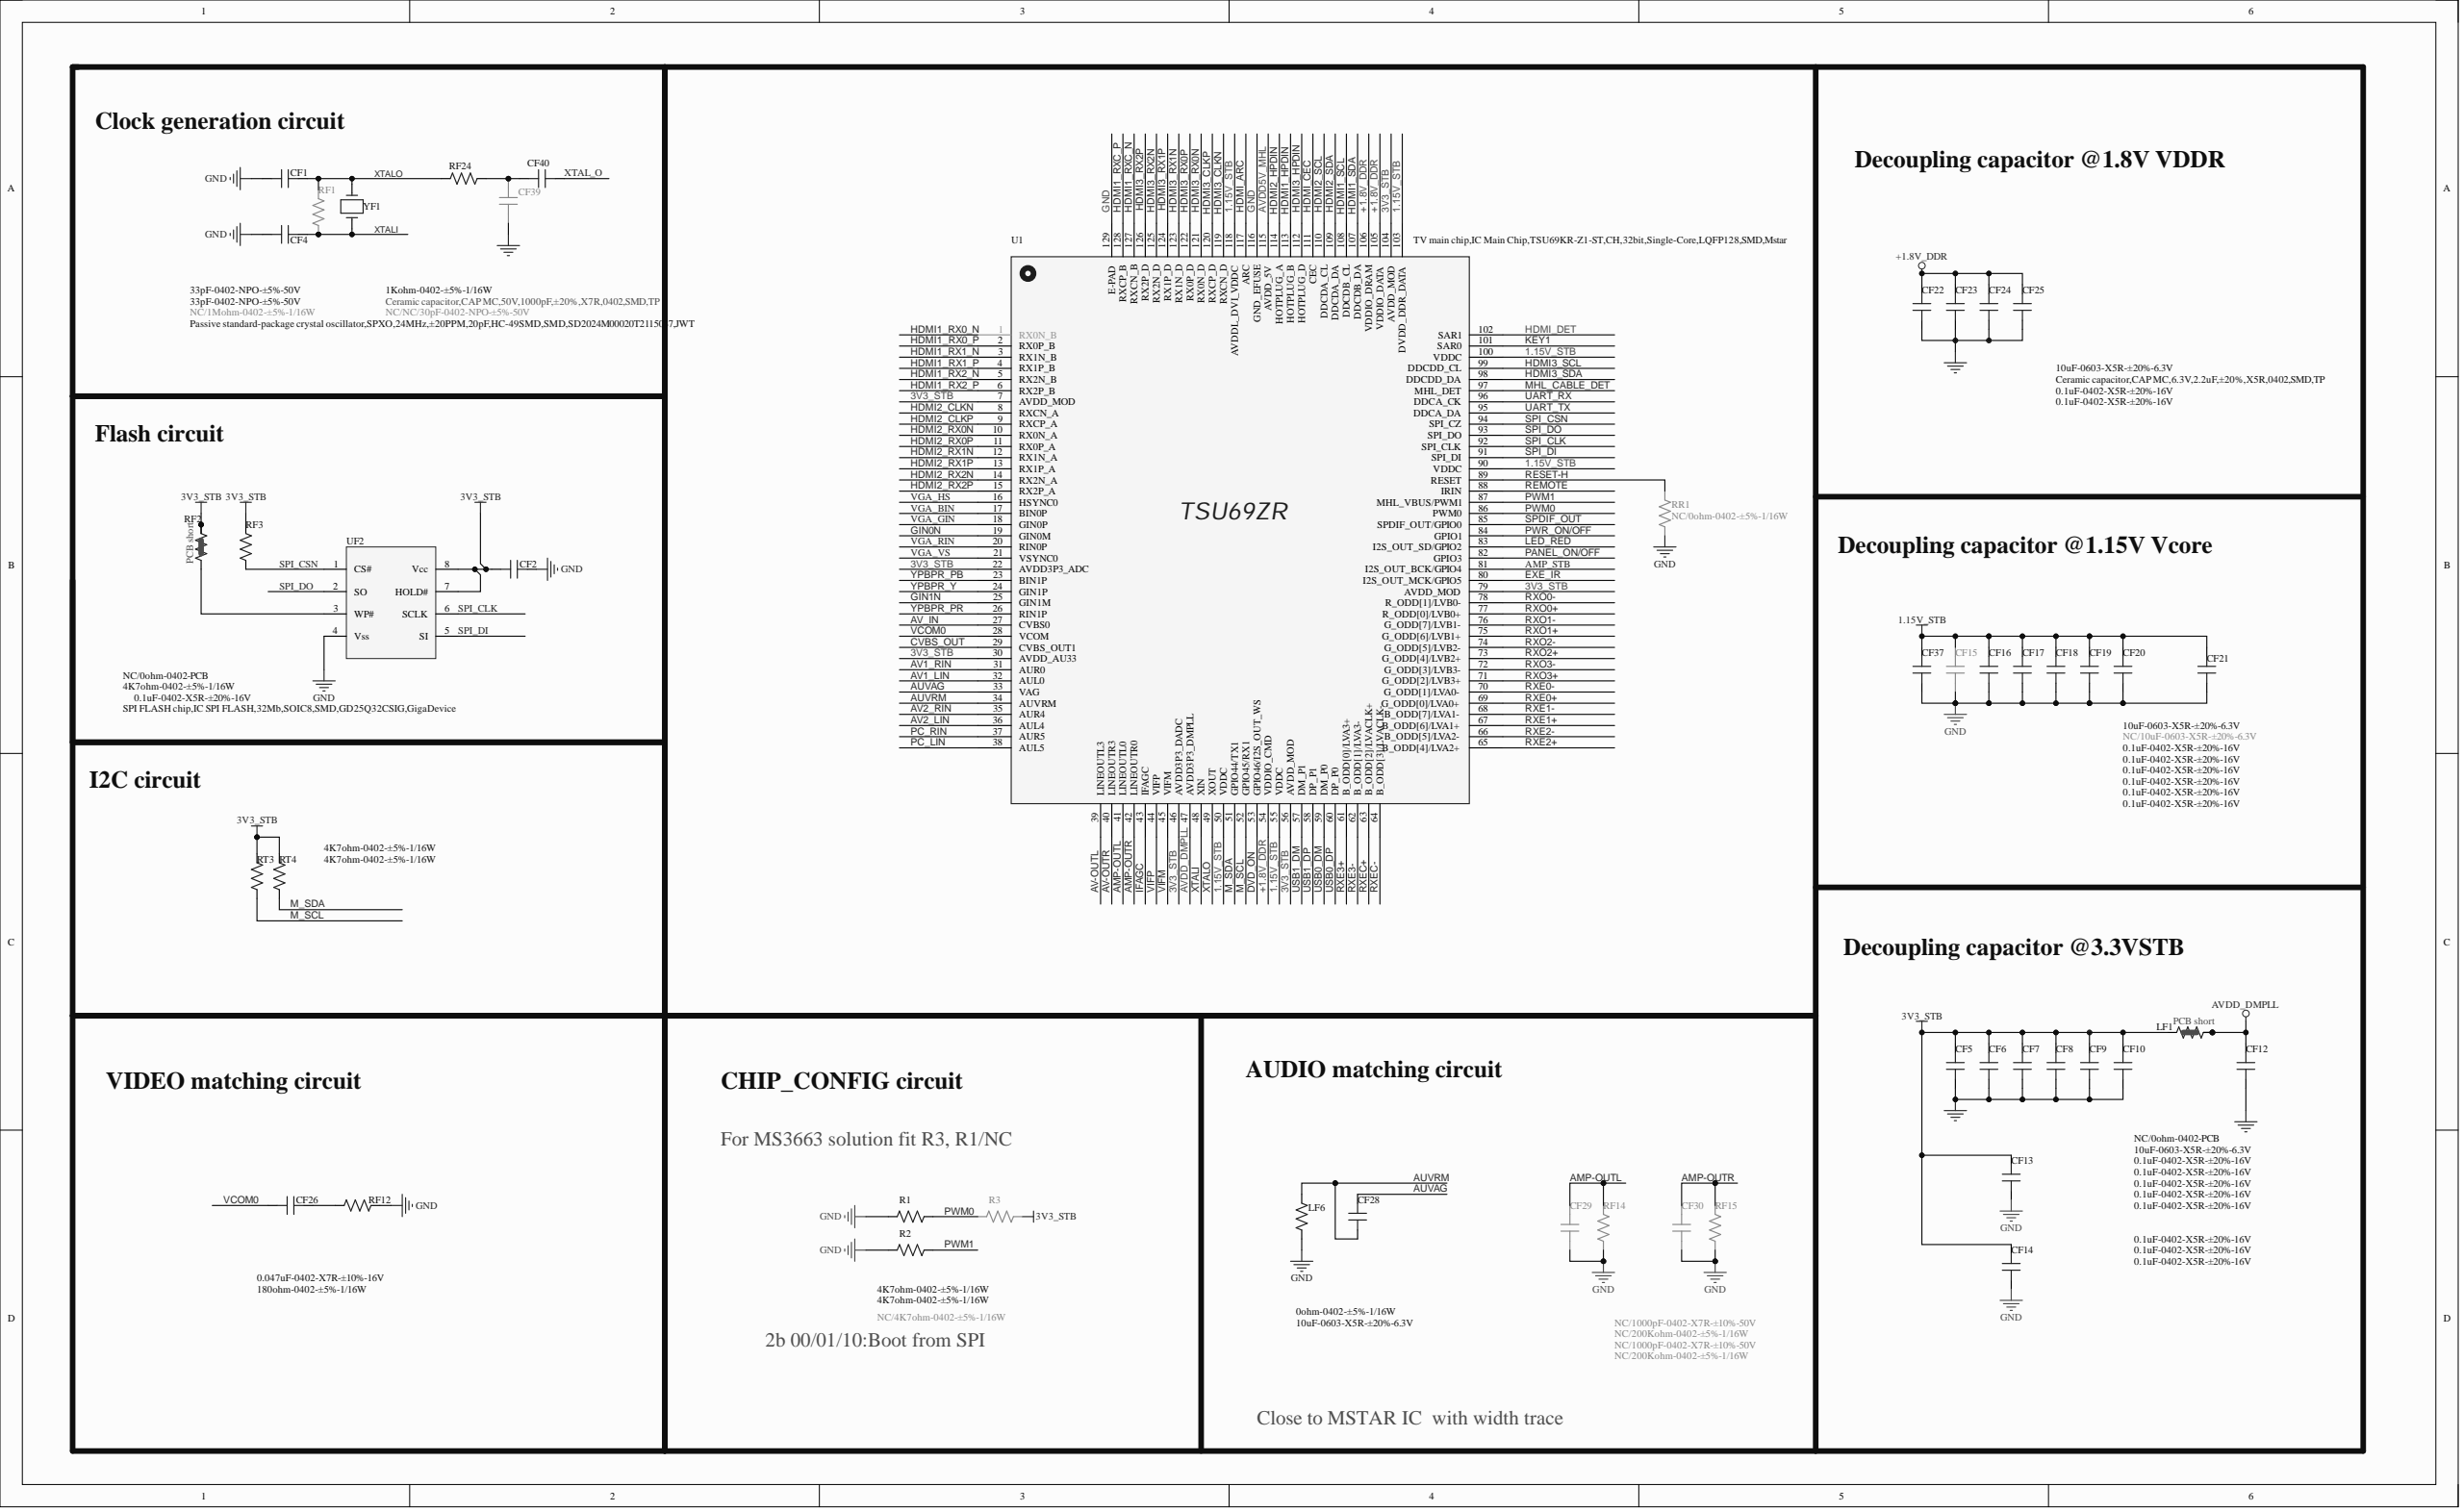Circuit board | Altium Designer | 574 parts | 274 nets | one sheet of the schematic
Parts on this sheet (reference | value | footprint):
CF1 | 33pF-0402-NPO-±5%-50V | C0402
CF2 | 0.1uF-0402-X5R-±20%-16V | C0402
CF4 | 33pF-0402-NPO-±5%-50V | C0402
CF5 | 10uF-0603-X5R-±20%-6.3V | C0603
CF6 | 0.1uF-0402-X5R-±20%-16V | C0402
CF7 | 0.1uF-0402-X5R-±20%-16V | C0402
CF8 | 0.1uF-0402-X5R-±20%-16V | C0402
CF9 | 0.1uF-0402-X5R-±20%-16V | C0402
CF10 | 0.1uF-0402-X5R-±20%-16V | C0402
CF12 | 0.1uF-0402-X5R-±20%-16V | C0402
CF13 | 0.1uF-0402-X5R-±20%-16V | C0402
CF14 | 0.1uF-0402-X5R-±20%-16V | C0402
CF15 | NC/10uF-0603-X5R-±20%-6.3V | C0603
CF16 | 0.1uF-0402-X5R-±20%-16V | C0402
CF17 | 0.1uF-0402-X5R-±20%-16V | C0402
CF18 | 0.1uF-0402-X5R-±20%-16V | C0402
CF19 | 0.1uF-0402-X5R-±20%-16V | C0402
CF20 | 0.1uF-0402-X5R-±20%-16V | C0402
CF21 | 0.1uF-0402-X5R-±20%-16V | C0402
CF22 | 10uF-0603-X5R-±20%-6.3V | C0603
CF23 | Ceramic capacitor,CAP MC,6.3V,2.2uF,±20%,X5R,0402,SMD,TP | C0402
CF24 | 0.1uF-0402-X5R-±20%-16V | C0402
CF25 | 0.1uF-0402-X5R-±20%-16V | C0402
CF26 | 0.047uF-0402-X7R-±10%-16V | C0402
CF28 | 10uF-0603-X5R-±20%-6.3V | C0603
CF29 | NC/1000pF-0402-X7R-±10%-50V | C0402
CF30 | NC/1000pF-0402-X7R-±10%-50V | C0402
CF37 | 10uF-0603-X5R-±20%-6.3V | C0603
CF39 | NC/NC/30pF-0402-NPO-±5%-50V | C0402
CF40 | Ceramic capacitor,CAP MC,50V,1000pF,±20%,X7R,0402,SMD,TP | C0402
LF1 | NC/0ohm-0402-PCB | R0402SC
LF6 | 0ohm-0402-±5%-1/16W | R0402
R3 | NC/4K7ohm-0402-±5%-1/16W | R0402
RF1 | NC/1Mohm-0402-±5%-1/16W | R0402
RF3 | 4K7ohm-0402-±5%-1/16W | R0402
RF12 | 180ohm-0402-±5%-1/16W | R0402
RF14 | NC/200Kohm-0402-±5%-1/16W | R0402
RF15 | NC/200Kohm-0402-±5%-1/16W | R0402
RF24 | 1Kohm-0402-±5%-1/16W | R0402
RR1 | NC/0ohm-0402-±5%-1/16W | R0402
RT3 | 4K7ohm-0402-±5%-1/16W | R0402
RT4 | 4K7ohm-0402-±5%-1/16W | R0402
U1 | TV main chip,IC Main Chip,TSU69KR-Z1-ST,CH,32bit,Single-Core,LQFP128,SMD,Mstar | QFP128/0.4-5
UF2 | SPI FLASH chip,IC SPI FLASH,32Mb,SOIC8,SMD,GD25Q32CSIG,GigaDevice | SOIC8
YF1 | Passive standard-package crystal oscillator,SPXO,24MHz,±20PPM,20pF,HC-49SMD,SMD,SD2024M00020T2115047,JWT | XTAL-S-1
Nets of these parts (net: part-pin ...):
YPBPR_Y: U1-24
XTALO: CF1-2 RF1-2 RF24-2 YF1-2 U1-49
XTALI: CF4-2 RF1-1 YF1-1 U1-48
XTAL_O: CF40-1
VIFP: U1-44
VIFM: U1-45
VGA_VS: U1-21
VGA_RIN: U1-20
VGA_HS: U1-16
VGA_GIN: U1-18
VGA_BIN: U1-17
VCOM0: CF26-1 U1-28
USB0_DP: U1-60
USB0_DM: U1-59
UART_TX: U1-95
UART_RX: U1-96
SPI_DO: UF2-2 U1-93
SPI_DI: UF2-5 U1-91
SPI_CSN: RF3-1 UF2-1 U1-94
SPI_CLK: UF2-6 U1-92
RXEC+: U1-63
RXE3+: U1-61
RXE2-: U1-66
RXE2+: U1-65
RXE1-: U1-68
RXE1+: U1-67
RXE0-: U1-70
RXE0+: U1-69
RESET-H: RR1-2 U1-89
REMOTE: U1-88
PWR_ON/OFF: U1-84
PWM1: U1-87
PWM0: R3-1 U1-86
PANEL_ON/OFF: U1-82
NetRF2_1: UF2-3
NetCF39_2: CF39-2 CF40-2 RF24-1
NetCF26_2: CF26-2 RF12-1
M_SDA: RT4-2 U1-51
M_SCL: RT3-2 U1-52
LED_RED: U1-83
KEY1: U1-101
IFAGC: U1-43
HDMI_DET: U1-102
HDMI_CEC: U1-111
HDMI_ARC: U1-117
HDMI1_SDA: U1-107
HDMI1_SCL: U1-108
HDMI1_RXC_P: U1-128
HDMI1_RXC_N: U1-127
HDMI1_RX2_P: U1-6
HDMI1_RX2_N: U1-5
HDMI1_RX1_P: U1-4
HDMI1_RX1_N: U1-3
HDMI1_RX0_P: U1-2
HDMI1_RX0_N: U1-1
HDMI1_HPDIN: U1-113
GND: CF1-1 CF2-1 CF4-1 CF5-2 CF6-1 CF7-1 CF8-1 CF9-1 CF10-1 CF12-1 CF13-1 CF14-1 CF15-2 CF16-1 CF17-1 CF18-1 CF19-1 CF20-1 CF21-1 CF22-2 CF23-1 CF24-1 CF25-1 CF29-2 CF30-2 CF37-2 CF39-1 LF6-1 RF12-2 RF14-1 RF15-1 RR1-1 UF2-4 U1-116 U1-129
GIN1N: U1-25
GIN0N: U1-19
EXE_IR: U1-80
CVBS_OUT: U1-29
AVDD_DMPLL: CF12-2 LF1-2 LF1-3 U1-47
AV_IN: U1-27
AV-OUTR: U1-40
AV-OUTL: U1-39
AV2_RIN: U1-35
AV2_LIN: U1-36
AV1_RIN: U1-31
AV1_LIN: U1-32
AUVRM: CF28-1 LF6-2 U1-34
AUVAG: CF28-2 U1-33
AMP_STB: U1-81
AMP-OUTR: CF30-1 RF15-2 U1-42
AMP-OUTL: CF29-1 RF14-2 U1-41
+1.8V_DDR: CF22-1 CF23-2 CF24-2 CF25-2 U1-54 U1-105 U1-106
3V3_STB: CF2-2 CF5-1 CF6-2 CF7-2 CF8-2 CF9-2 CF10-2 CF13-2 CF14-2 LF1-1 R3-2 RF3-2 RT3-1 RT4-1 UF2-7 UF2-8 U1-7 U1-22 U1-30 U1-46 U1-56 U1-79 U1-104
1.15V_STB: CF15-1 CF16-2 CF17-2 CF18-2 CF19-2 CF20-2 CF21-2 CF37-1 U1-50 U1-55 U1-90 U1-100 U1-103 U1-118